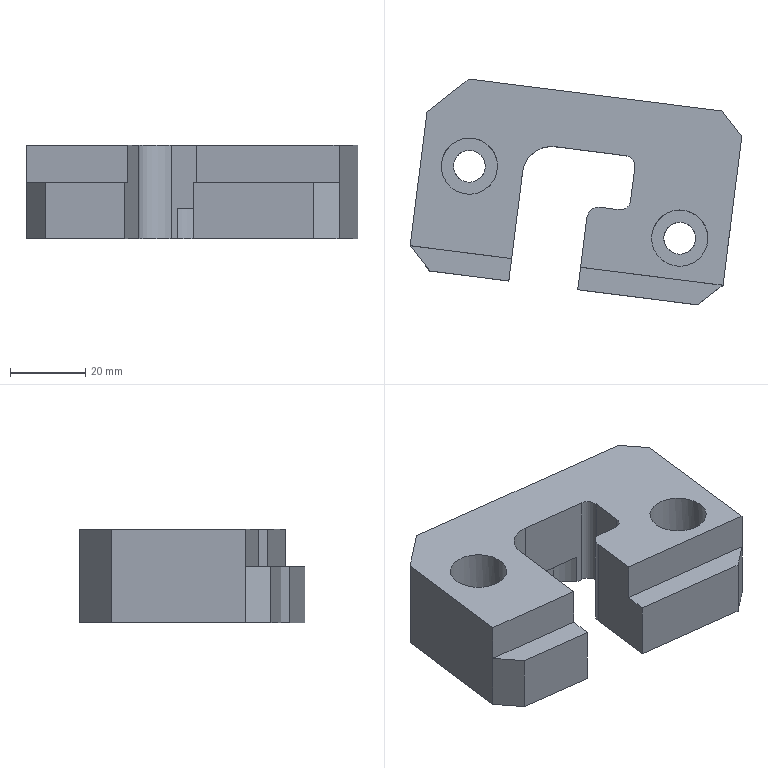Part | STEP file | gslz 2016.10.28-13_id1702_x_t | 1 solid | 34 faces | box 88.351 x 60.113 x 25 mm | volume 76522 mm3 | plane 24 | cylinder 10 | commonest cylinder face diameters 5.5 x2 8.5 x2 14 x2 15 x2 6.5 x1 15.5 x1